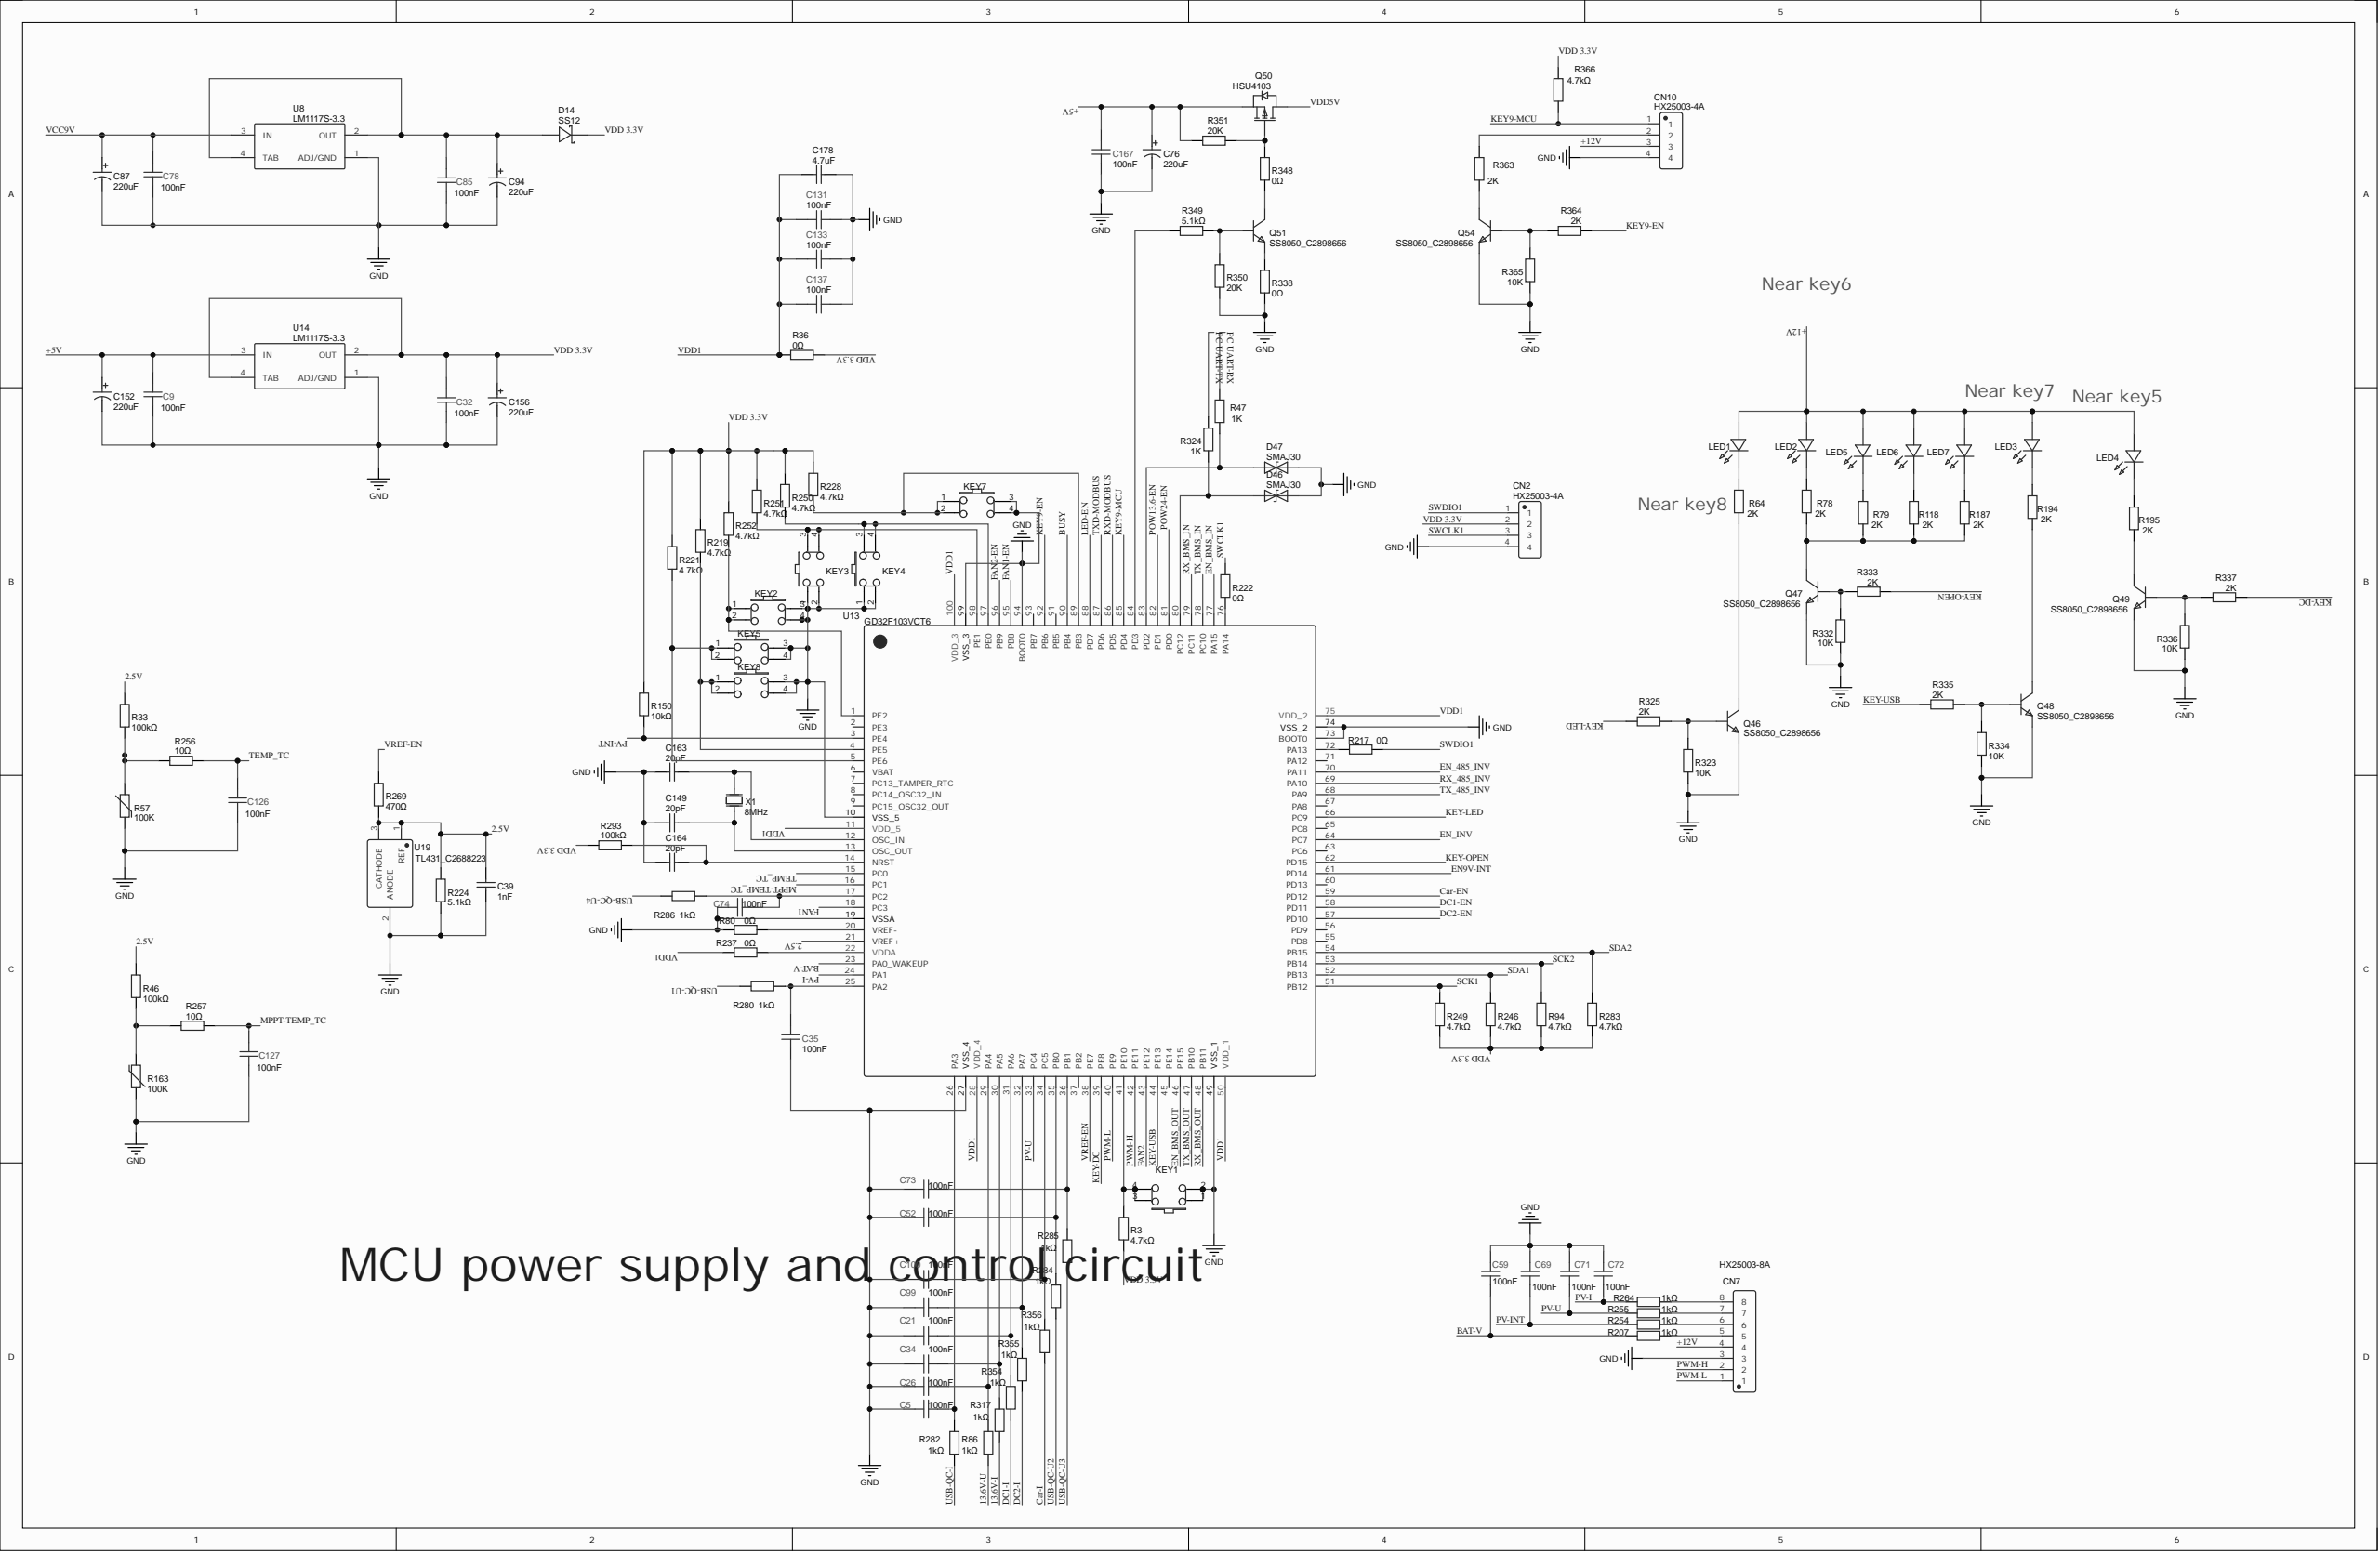Circuit board | Altium Designer | 694 parts | 423 nets | one sheet of the schematic
Parts on this sheet (reference | value | footprint):
C5 | 100nF | C0603
C9 | 100nF | C0603
C21 | 100nF | C0603
C26 | 100nF | C0603
C32 | 100nF | C0603
C34 | 100nF | C0603
C35 | 100nF | C0603
C39 | 1nF | C0603
C52 | 100nF | C0603
C59 | 100nF | C0603
C69 | 100nF | C0603
C71 | 100nF | C0603
C72 | 100nF | C0603
C73 | 100nF | C0603
C74 | 100nF | C0603
C76 | 220uF | CAP-TH_BD6.3-P2.50-D1.0-FD
C78 | 100nF | C0603
C85 | 100nF | C0603
C87 | 220uF | CAP-TH_BD6.3-P2.50-D1.0-FD
C94 | 220uF | CAP-TH_BD6.3-P2.50-D1.0-FD
C99 | 100nF | C0603
C100 | 100nF | C0603
C126 | 100nF | C0603
C127 | 100nF | C0603
C131 | 100nF | C0603
C133 | 100nF | C0603
C137 | 100nF | C0603
C149 | 20pF | C0603
C152 | 220uF | CAP-TH_BD6.3-P2.50-D1.0-FD
C156 | 220uF | CAP-TH_BD6.3-P2.50-D1.0-FD
C163 | 20pF | C0603
C164 | 20pF | C0603
C167 | 100nF | C0603
C178 | 4.7uF | C0805
CN2 | HX25003-4A | CONN-TH_4P-P2.50_HX25003-4A
CN7 | HX25003-8A | CONN-TH_8P-P2.50_HX25003-8A
CN10 | HX25003-4A | CONN-TH_4P-P2.50_HX25003-4A
D14 | SS12 | SMA_L4.3-W2.6-LS5.2-RD
D46 | SMAJ30 | SMA_L4.3-W2.5-LS5.0-BI
D47 | SMAJ30 | SMA_L4.3-W2.5-LS5.0-BI
KEY1 | 4-1437565-2 | SW-SMD_4P-L6.0-W6.0-P4.50-LS8.6
KEY2 | 4-1437565-2 | SW-SMD_4P-L6.0-W6.0-P4.50-LS8.6
KEY3 | 4-1437565-2 | SW-SMD_4P-L6.0-W6.0-P4.50-LS8.6
KEY4 | 4-1437565-2 | SW-SMD_4P-L6.0-W6.0-P4.50-LS8.6
KEY5 | 4-1437565-2 | SW-SMD_4P-L6.0-W6.0-P4.50-LS8.6
KEY7 | 4-1437565-2 | SW-SMD_4P-L6.0-W6.0-P4.50-LS8.6
KEY8 | 4-1437565-2 | SW-SMD_4P-L6.0-W6.0-P4.50-LS8.6
LED1 | LED-0603_R | LED0603_RED
LED2 | LED-0603_R | LED0603_RED
LED3 | LED-0603_R | LED0603_RED
LED4 | LED-0603_R | LED0603_RED
LED5 | LED-0603_R | LED0603_RED
LED6 | LED-0603_R | LED0603_RED
LED7 | LED-0603_R | LED0603_RED
Q46 | SS8050_C2898656 | SOT-23-3_L2.9-W1.3-P1.90-LS2.4-BR
Q47 | SS8050_C2898656 | SOT-23-3_L2.9-W1.3-P1.90-LS2.4-BR
Q48 | SS8050_C2898656 | SOT-23-3_L2.9-W1.3-P1.90-LS2.4-BR
Q49 | SS8050_C2898656 | SOT-23-3_L2.9-W1.3-P1.90-LS2.4-BR
Q50 | HSU4103 | TO-252-2_L6.6-W6.1-P4.57-LS9.9-BR
Q51 | SS8050_C2898656 | SOT-23-3_L2.9-W1.3-P1.90-LS2.4-BR
Q54 | SS8050_C2898656 | SOT-23-3_L2.9-W1.3-P1.90-LS2.4-BR
R3 | 4.7kΩ | R0603
R33 | 100kΩ | R0603
R36 | 0Ω | R0603
R46 | 100kΩ | R0603
R47 | 1K | R0603
R57 | 100K | NTC
R64 | 2K | R0603
R78 | 2K | R0603
R79 | 2K | R0603
R80 | 0Ω | R0603
R86 | 1kΩ | R0603
R94 | 4.7kΩ | R0603
R118 | 2K | R0603
R150 | 10kΩ | R0603
R163 | 100K | NTC
R187 | 2K | R0603
R194 | 2K | R0603
R195 | 2K | R0603
R207 | 1kΩ | R0603
R217 | 0Ω | R0603
R219 | 4.7kΩ | R0603
R221 | 4.7kΩ | R0603
R222 | 0Ω | R0603
R224 | 5.1kΩ | R0603
R228 | 4.7kΩ | R0603
R237 | 0Ω | R0603
R246 | 4.7kΩ | R0603
R249 | 4.7kΩ | R0603
R250 | 4.7kΩ | R0603
R251 | 4.7kΩ | R0603
R252 | 4.7kΩ | R0603
R254 | 1kΩ | R0603
R255 | 1kΩ | R0603
R256 | 10Ω | R0603
R257 | 10Ω | R0603
R264 | 1kΩ | R0603
R269 | 470Ω | R0603
R280 | 1kΩ | R0603
R282 | 1kΩ | R0603
R283 | 4.7kΩ | R0603
R284 | 1kΩ | R0603
R285 | 1kΩ | R0603
R286 | 1kΩ | R0603
R293 | 100kΩ | R0603
R317 | 1kΩ | R0603
R323 | 10K | R0603
R324 | 1K | R0603
R325 | 2K | R0603
R332 | 10K | R0603
R333 | 2K | R0603
R334 | 10K | R0603
R335 | 2K | R0603
R336 | 10K | R0603
R337 | 2K | R0603
R338 | 0Ω | R0603
R348 | 0Ω | R0603
R349 | 5.1kΩ | R0603
R350 | 20K | R0603
R351 | 20K | R0603
R354 | 1kΩ | R0603
R355 | 1kΩ | R0603
R356 | 1kΩ | R0603
R363 | 2K | R0603
R364 | 2K | R0603
R365 | 10K | R0603
R366 | 4.7kΩ | R0603
U8 | LM1117S-3.3 | SOT-223-3_L6.5-W3.4-P2.30-LS7.0-BR
U13 | GD32F103VCT6 | LQFP-100_L14.0-W14.0-P0.50-LS16.0-BL
U14 | LM1117S-3.3 | SOT-223-3_L6.5-W3.4-P2.30-LS7.0-BR
U19 | TL431_C2688223 | SOT-23-3_L2.9-W1.6-P1.90-LS2.8-BR-CW
X1 | 8MHz | HC-49S_L11.4-W4.8
Nets of these parts (net: part-pin ...):
VREF-EN: R269-2 U13-38
VDD 3.3V: C32-2 C156-1 CN2-2 D14-1 R3-1 R36-1 R94-1 R150-2 R219-2 R221-2 R228-2 R246-1 R249-1 R250-2 R251-2 R252-2 R283-1 R293-2 R366-2 U14-2 U14-4
VDD5V: Q50-3
VDD1: C131-2 C133-2 C137-2 C178-1 R36-2 R237-1 U13-11 U13-28 U13-50 U13-75 U13-100
VCC9V: C78-2 C87-1 U8-3
USB-QC-U4: R286-1
USB-QC-U3: R285-1
USB-QC-U2: R284-2
USB-QC-U1: R280-1
USB-QC-I: R282-2
TXD-MODBUS: U13-87
TX_BMS_IN: U13-78
TX_485_INV: U13-68
TEMP_TC: C126-2 R256-2 U13-15
SWDIO1: CN2-1 R217-2
SWCLK1: CN2-3 R222-2
SDA2: R283-2 U13-54
SDA1: R246-2 U13-52
SCK2: R94-2 U13-53
SCK1: R249-2 U13-51
RXD-MODBUS: U13-86
RX_BMS_IN: U13-79
RX_485_INV: U13-69
PWM-L: CN7-1 U13-40
PWM-H: CN7-2 U13-42
PV-U: C71-2 R255-1 U13-33
PV-INT: C69-2 R150-1 R254-1 U13-3
PV-I: C72-2 R264-1 U13-24
POW24-EN: U13-81
POW13.6-EN: U13-82
PC UART-TX: R324-1
PC UART-RX: R47-1
NetR349_2: R349-2 U13-84
NetR237_2: R237-2 U13-22
NetR222_1: R222-1 U13-76
NetR217_1: R217-1 U13-72
NetR80_2: R80-2 U13-20
NetR46_1: R46-1 R163-1 R257-1
NetR33_1: R33-1 R57-2 R256-1
NetQ54_3: Q54-3 R363-2
NetQ54_1: Q54-1 R364-2 R365-1
NetQ51_3: Q51-3 R348-1
NetQ51_2: Q51-2 R338-2
NetQ51_1: Q51-1 R349-1 R350-2
NetQ50_1: Q50-1 R348-2 R351-2
NetQ49_3: Q49-3 R195-2
NetQ49_1: Q49-1 R336-1 R337-2
NetQ48_3: Q48-3 R194-2
NetQ48_1: Q48-1 R334-1 R335-2
NetQ47_3: Q47-3 R78-2 R79-2 R118-2 R187-2
NetQ47_1: Q47-1 R332-1 R333-2
NetQ46_3: Q46-3 R64-2
NetQ46_1: Q46-1 R323-1 R325-2
NetLED7_2: LED7-2 R187-1
NetLED6_2: LED6-2 R118-1
NetLED5_2: LED5-2 R79-1
NetLED4_2: LED4-2 R195-1
NetLED3_2: LED3-2 R194-1
NetLED2_2: LED2-2 R78-1
NetLED1_2: LED1-2 R64-1
NetKEY8_1: KEY8-1 KEY8-2 R219-1 U13-4
NetKEY7_1: KEY7-1 KEY7-2 R228-1 U13-89
NetKEY5_1: KEY5-1 KEY5-2 R221-1 U13-5
NetKEY4_3: KEY4-3 KEY4-4 R250-1 U13-97
NetKEY3_3: KEY3-3 KEY3-4 R251-1 U13-98
NetKEY2_1: KEY2-1 KEY2-2 R252-1 U13-1
NetKEY1_3: KEY1-3 KEY1-4 R3-2 U13-41
NetD47_2: D47-2 R47-2 U13-83
NetD46_2: D46-2 R324-2 U13-80
NetCN10_2: CN10-2 R363-1
NetCN7_8: CN7-8 R264-2
NetCN7_7: CN7-7 R255-2
NetCN7_6: CN7-6 R254-2
NetCN7_5: CN7-5 R207-2
NetC164_2: C164-2 R293-1 U13-14
NetC163_2: C163-2 X1-2 U13-12
NetC149_2: C149-2 X1-1 U13-13
NetC100_2: C100-2 R356-1 U13-34
NetC99_2: C99-2 R355-1 U13-32
NetC85_2: C85-2 C94-1 D14-2 U8-2 U8-4
NetC74_1: C74-1 R286-2 U13-17
NetC73_1: C73-1 R285-2 U13-36
NetC52_1: C52-1 R284-1 U13-35
NetC35_2: C35-2 R280-2 U13-25
NetC34_2: C34-2 R317-1 U13-30
NetC26_1: C26-1 R86-1 U13-29
NetC21_2: C21-2 R354-1 U13-31
NetC5_1: C5-1 R282-1 U13-26
MPPT-TEMP_TC: C127-2 R257-2 U13-16
LED-EN: U13-88
KEY-USB: R335-1 U13-44
KEY-OPEN: R333-1 U13-62
KEY-LED: R325-1 U13-66
KEY-DC: R337-1 U13-39
KEY9-MCU: CN10-1 R366-1 U13-85
KEY9-EN: R364-1 U13-92
GND: C5-2 C9-1 C21-1 C26-2 C32-1 C34-1 C35-1 C39-1 C52-2 C59-1 C69-1 C71-1 C72-1 C73-2 C74-2 C76-2 C78-1 C85-1 C87-2 C94-2 C99-1 C100-1 C126-1 C127-1 C131-1 C133-1 C137-1 C149-1 C152-2 C156-2 C163-1 C164-1 C167-2 C178-2 CN2-4 CN7-3 CN10-4 D46-1 D47-1 KEY1-1 KEY1-2 KEY2-3 KEY2-4 KEY3-1 KEY3-2 KEY4-1 KEY4-2 KEY5-3 KEY5-4 KEY7-3 KEY7-4 KEY8-3 KEY8-4 Q46-2 Q47-2 Q48-2 Q49-2 Q54-2 R57-1 R80-1 R163-2 R224-2 R323-2 R332-2 R334-2 R336-2 R338-1 R350-1 R365-2 U8-1 U14-1 U19-2 U13-10 U13-19 U13-27 U13-49 U13-73 U13-74 U13-94 U13-99
FAN1-EN: U13-95
EN_INV: U13-64
EN_BMS_IN: U13-77
EN_485_INV: U13-70
EN9V-INT: U13-61
DC2-I: R355-2
DC2-EN: U13-57
DC1-I: R354-2
DC1-EN: U13-58
Car-I: R356-2
Car-EN: U13-59
BUSY: U13-90
BAT-V: C59-2 R207-1 U13-23
+12V: CN7-4 CN10-3 LED1-1 LED2-1 LED3-1 LED4-1 LED5-1 LED6-1 LED7-1
+5V: C9-2 C76-1 C152-1 C167-1 Q50-2 R351-1 U14-3
13.6V-U: R86-2
13.6V-I: R317-2
2.5V: C39-2 R33-2 R46-2 R224-1 R269-1 U19-1 U19-3 U13-21